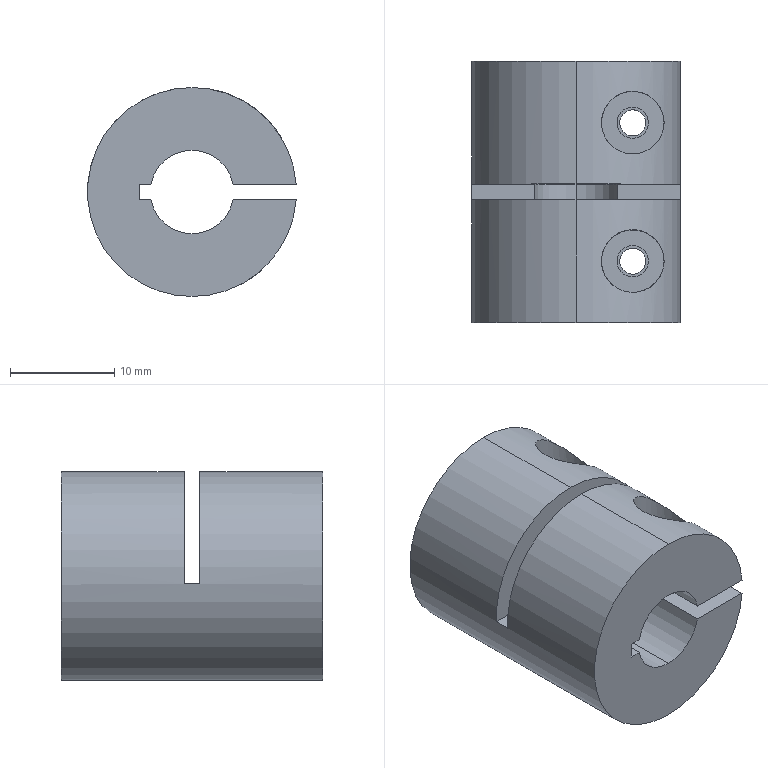Part | SolidWorks | features ICE 4, Extrusion 1, HoleWzd 1 | 1 solid | 34 faces | box 19.972 x 25 x 20 mm | volume 5780 mm3 | cylinder 20 | plane 14 | commonest cylinder face diameters 2.5 x4 3 x4 6 x4 8 x4 20 x4
STEP:
#1=CARTESIAN_POINT('',(4.179,19.125,-9.085));
#2=VERTEX_POINT('',#1);
#3=CARTESIAN_POINT('',(6.679,19.125,-7.442));
#4=VERTEX_POINT('',#3);
#5=CARTESIAN_POINT('',(4.179,19.125,-9.085));
#6=CARTESIAN_POINT('',(4.179,19.034,-9.085));
#7=CARTESIAN_POINT('',(4.189,18.945,-9.08));
#8=CARTESIAN_POINT('',(4.227,18.77,-9.063));
#9=CARTESIAN_POINT('',(4.256,18.684,-9.049));
#10=CARTESIAN_POINT('',(4.33,18.524,-9.014));
#11=CARTESIAN_POINT('',(4.375,18.448,-8.992));
#12=CARTESIAN_POINT('',(4.478,18.309,-8.941));
#13=CARTESIAN_POINT('',(4.536,18.246,-8.912));
#14=CARTESIAN_POINT('',(4.725,18.078,-8.814));
#15=CARTESIAN_POINT('',(4.87,17.996,-8.736));
#16=CARTESIAN_POINT('',(5.169,17.892,-8.562));
#17=CARTESIAN_POINT('',(5.323,17.87,-8.467));
#18=CARTESIAN_POINT('',(5.625,17.881,-8.27));
#19=CARTESIAN_POINT('',(5.772,17.914,-8.168));
#20=CARTESIAN_POINT('',(6.047,18.028,-7.966));
#21=CARTESIAN_POINT('',(6.174,18.11,-7.867));
#22=CARTESIAN_POINT('',(6.344,18.27,-7.73));
#23=CARTESIAN_POINT('',(6.396,18.329,-7.687));
#24=CARTESIAN_POINT('',(6.491,18.46,-7.608));
#25=CARTESIAN_POINT('',(6.533,18.533,-7.571));
#26=CARTESIAN_POINT('',(6.638,18.765,-7.48));
#27=CARTESIAN_POINT('',(6.679,18.943,-7.442));
#28=CARTESIAN_POINT('',(6.679,19.125,-7.442));
#29=B_SPLINE_CURVE_WITH_KNOTS('',3,(#5,#6,#7,#8,#9,#10,#11,#12,#13,#14,#15,#16,#17,#18,#19,#20,#21,#22,#23,#24,#25,#26,#27,#28),.UNSPECIFIED.,.F.,.F.,(4,2,2,2,2,2,2,2,2,2,2,4),(0.004311,0.00458,0.004848,0.005117,0.005385,0.005923,0.00646,0.006997,0.007534,0.007803,0.008071,0.008608),.UNSPECIFIED.);
#30=EDGE_CURVE('',#2,#4,#29,.T.);
#31=ORIENTED_EDGE('',*,*,#30,.F.);
#32=CARTESIAN_POINT('',(4.179,19.125,-0.75));
#33=VERTEX_POINT('',#32);
#34=CARTESIAN_POINT('',(4.179,19.125,-0.75));
#35=DIRECTION('',(0.,0.,1.));
#36=VECTOR('',#35,1000.);
#37=LINE('',#34,#36);
#38=EDGE_CURVE('',#2,#33,#37,.T.);
#39=ORIENTED_EDGE('',*,*,#38,.T.);
#40=CARTESIAN_POINT('',(6.679,19.125,-0.75));
#41=VERTEX_POINT('',#40);
#42=CARTESIAN_POINT('',(5.429,19.125,-0.75));
#43=DIRECTION('',(0.,0.,1.));
#44=DIRECTION('',(1.,0.,0.));
#45=AXIS2_PLACEMENT_3D('',#42,#43,#44);
#46=CIRCLE('',#45,1.25);
#47=EDGE_CURVE('',#33,#41,#46,.T.);
#48=ORIENTED_EDGE('',*,*,#47,.T.);
#49=CARTESIAN_POINT('',(6.679,19.125,-0.75));
#50=DIRECTION('',(0.,0.,1.));
#51=VECTOR('',#50,1000.);
#52=LINE('',#49,#51);
#53=EDGE_CURVE('',#4,#41,#52,.T.);
#54=ORIENTED_EDGE('',*,*,#53,.F.);
#55=EDGE_LOOP('',(#31,#39,#48,#54));
#56=FACE_OUTER_BOUND('',#55,.T.);
#57=CARTESIAN_POINT('',(5.429,19.125,-0.75));
#58=DIRECTION('',(0.,0.,1.));
#59=DIRECTION('',(1.,0.,0.));
#60=AXIS2_PLACEMENT_3D('',#57,#58,#59);
#61=CYLINDRICAL_SURFACE('',#60,1.25);
#62=ADVANCED_FACE('',(#56),#61,.F.);
#63=CARTESIAN_POINT('',(4.179,5.875,-9.085));
#64=VERTEX_POINT('',#63);
#65=CARTESIAN_POINT('',(6.679,5.875,-7.442));
#66=VERTEX_POINT('',#65);
#67=CARTESIAN_POINT('',(4.179,5.875,-9.085));
#68=CARTESIAN_POINT('',(4.179,5.784,-9.085));
#69=CARTESIAN_POINT('',(4.189,5.695,-9.08));
#70=CARTESIAN_POINT('',(4.227,5.52,-9.063));
#71=CARTESIAN_POINT('',(4.256,5.434,-9.049));
#72=CARTESIAN_POINT('',(4.33,5.274,-9.014));
#73=CARTESIAN_POINT('',(4.375,5.198,-8.992));
#74=CARTESIAN_POINT('',(4.478,5.059,-8.941));
#75=CARTESIAN_POINT('',(4.536,4.996,-8.912));
#76=CARTESIAN_POINT('',(4.725,4.828,-8.814));
#77=CARTESIAN_POINT('',(4.87,4.746,-8.736));
#78=CARTESIAN_POINT('',(5.169,4.642,-8.562));
#79=CARTESIAN_POINT('',(5.323,4.62,-8.467));
#80=CARTESIAN_POINT('',(5.625,4.631,-8.27));
#81=CARTESIAN_POINT('',(5.772,4.664,-8.168));
#82=CARTESIAN_POINT('',(6.047,4.778,-7.966));
#83=CARTESIAN_POINT('',(6.174,4.86,-7.867));
#84=CARTESIAN_POINT('',(6.344,5.02,-7.73));
#85=CARTESIAN_POINT('',(6.396,5.079,-7.687));
#86=CARTESIAN_POINT('',(6.491,5.21,-7.608));
#87=CARTESIAN_POINT('',(6.533,5.283,-7.571));
#88=CARTESIAN_POINT('',(6.638,5.515,-7.48));
#89=CARTESIAN_POINT('',(6.679,5.693,-7.442));
#90=CARTESIAN_POINT('',(6.679,5.875,-7.442));
#91=B_SPLINE_CURVE_WITH_KNOTS('',3,(#67,#68,#69,#70,#71,#72,#73,#74,#75,#76,#77,#78,#79,#80,#81,#82,#83,#84,#85,#86,#87,#88,#89,#90),.UNSPECIFIED.,.F.,.F.,(4,2,2,2,2,2,2,2,2,2,2,4),(0.004311,0.00458,0.004848,0.005117,0.005385,0.005923,0.00646,0.006997,0.007534,0.007803,0.008071,0.008608),.UNSPECIFIED.);
#92=EDGE_CURVE('',#64,#66,#91,.T.);
#93=ORIENTED_EDGE('',*,*,#92,.F.);
#94=CARTESIAN_POINT('',(4.179,5.875,-0.75));
#95=VERTEX_POINT('',#94);
#96=CARTESIAN_POINT('',(4.179,5.875,-0.75));
#97=DIRECTION('',(0.,0.,1.));
#98=VECTOR('',#97,1000.);
#99=LINE('',#96,#98);
#100=EDGE_CURVE('',#64,#95,#99,.T.);
#101=ORIENTED_EDGE('',*,*,#100,.T.);
#102=CARTESIAN_POINT('',(6.679,5.875,-0.75));
#103=VERTEX_POINT('',#102);
#104=CARTESIAN_POINT('',(5.429,5.875,-0.75));
#105=DIRECTION('',(0.,0.,1.));
#106=DIRECTION('',(1.,0.,0.));
#107=AXIS2_PLACEMENT_3D('',#104,#105,#106);
#108=CIRCLE('',#107,1.25);
#109=EDGE_CURVE('',#95,#103,#108,.T.);
#110=ORIENTED_EDGE('',*,*,#109,.T.);
#111=CARTESIAN_POINT('',(6.679,5.875,-0.75));
#112=DIRECTION('',(0.,0.,1.));
#113=VECTOR('',#112,1000.);
#114=LINE('',#111,#113);
#115=EDGE_CURVE('',#66,#103,#114,.T.);
#116=ORIENTED_EDGE('',*,*,#115,.F.);
#117=EDGE_LOOP('',(#93,#101,#110,#116));
#118=FACE_OUTER_BOUND('',#117,.T.);
#119=CARTESIAN_POINT('',(5.429,5.875,-0.75));
#120=DIRECTION('',(0.,0.,1.));
#121=DIRECTION('',(1.,0.,0.));
#122=AXIS2_PLACEMENT_3D('',#119,#120,#121);
#123=CYLINDRICAL_SURFACE('',#122,1.25);
#124=ADVANCED_FACE('',(#118),#123,.F.);
#125=CARTESIAN_POINT('',(3.929,19.125,0.75));
#126=VERTEX_POINT('',#125);
#127=CARTESIAN_POINT('',(6.929,19.125,0.75));
#128=VERTEX_POINT('',#127);
#129=CARTESIAN_POINT('',(5.429,19.125,0.75));
#130=DIRECTION('',(0.,0.,1.));
#131=DIRECTION('',(1.,0.,0.));
#132=AXIS2_PLACEMENT_3D('',#129,#130,#131);
#133=CIRCLE('',#132,1.5);
#134=EDGE_CURVE('',#126,#128,#133,.T.);
#135=ORIENTED_EDGE('',*,*,#134,.F.);
#136=CARTESIAN_POINT('',(3.929,19.125,4.));
#137=VERTEX_POINT('',#136);
#138=CARTESIAN_POINT('',(3.929,19.125,0.));
#139=DIRECTION('',(0.,0.,1.));
#140=VECTOR('',#139,1000.);
#141=LINE('',#138,#140);
#142=EDGE_CURVE('',#126,#137,#141,.T.);
#143=ORIENTED_EDGE('',*,*,#142,.T.);
#144=CARTESIAN_POINT('',(6.929,19.125,4.));
#145=VERTEX_POINT('',#144);
#146=CARTESIAN_POINT('',(5.429,19.125,4.));
#147=DIRECTION('',(0.,0.,1.));
#148=DIRECTION('',(1.,0.,0.));
#149=AXIS2_PLACEMENT_3D('',#146,#147,#148);
#150=CIRCLE('',#149,1.5);
#151=EDGE_CURVE('',#137,#145,#150,.T.);
#152=ORIENTED_EDGE('',*,*,#151,.T.);
#153=CARTESIAN_POINT('',(6.929,19.125,0.));
#154=DIRECTION('',(0.,0.,1.));
#155=VECTOR('',#154,1000.);
#156=LINE('',#153,#155);
#157=EDGE_CURVE('',#128,#145,#156,.T.);
#158=ORIENTED_EDGE('',*,*,#157,.F.);
#159=EDGE_LOOP('',(#135,#143,#152,#158));
#160=FACE_OUTER_BOUND('',#159,.T.);
#161=CARTESIAN_POINT('',(5.429,19.125,0.));
#162=DIRECTION('',(0.,0.,1.));
#163=DIRECTION('',(1.,0.,0.));
#164=AXIS2_PLACEMENT_3D('',#161,#162,#163);
#165=CYLINDRICAL_SURFACE('',#164,1.5);
#166=ADVANCED_FACE('',(#160),#165,.F.);
#167=CARTESIAN_POINT('',(3.929,5.875,0.75));
#168=VERTEX_POINT('',#167);
#169=CARTESIAN_POINT('',(6.929,5.875,0.75));
#170=VERTEX_POINT('',#169);
#171=CARTESIAN_POINT('',(5.429,5.875,0.75));
#172=DIRECTION('',(0.,0.,1.));
#173=DIRECTION('',(1.,0.,0.));
#174=AXIS2_PLACEMENT_3D('',#171,#172,#173);
#175=CIRCLE('',#174,1.5);
#176=EDGE_CURVE('',#168,#170,#175,.T.);
#177=ORIENTED_EDGE('',*,*,#176,.F.);
#178=CARTESIAN_POINT('',(3.929,5.875,4.));
#179=VERTEX_POINT('',#178);
#180=CARTESIAN_POINT('',(3.929,5.875,0.));
#181=DIRECTION('',(0.,0.,1.));
#182=VECTOR('',#181,1000.);
#183=LINE('',#180,#182);
#184=EDGE_CURVE('',#168,#179,#183,.T.);
#185=ORIENTED_EDGE('',*,*,#184,.T.);
#186=CARTESIAN_POINT('',(6.929,5.875,4.));
#187=VERTEX_POINT('',#186);
#188=CARTESIAN_POINT('',(5.429,5.875,4.));
#189=DIRECTION('',(0.,0.,1.));
#190=DIRECTION('',(1.,0.,0.));
#191=AXIS2_PLACEMENT_3D('',#188,#189,#190);
#192=CIRCLE('',#191,1.5);
#193=EDGE_CURVE('',#179,#187,#192,.T.);
#194=ORIENTED_EDGE('',*,*,#193,.T.);
#195=CARTESIAN_POINT('',(6.929,5.875,0.));
#196=DIRECTION('',(0.,0.,1.));
#197=VECTOR('',#196,1000.);
#198=LINE('',#195,#197);
#199=EDGE_CURVE('',#170,#187,#198,.T.);
#200=ORIENTED_EDGE('',*,*,#199,.F.);
#201=EDGE_LOOP('',(#177,#185,#194,#200));
#202=FACE_OUTER_BOUND('',#201,.T.);
#203=CARTESIAN_POINT('',(5.429,5.875,0.));
#204=DIRECTION('',(0.,0.,1.));
#205=DIRECTION('',(1.,0.,0.));
#206=AXIS2_PLACEMENT_3D('',#203,#204,#205);
#207=CYLINDRICAL_SURFACE('',#206,1.5);
#208=ADVANCED_FACE('',(#202),#207,.F.);
#209=CARTESIAN_POINT('',(2.429,5.875,4.));
#210=VERTEX_POINT('',#209);
#211=CARTESIAN_POINT('',(8.429,5.875,4.));
#212=VERTEX_POINT('',#211);
#213=CARTESIAN_POINT('',(5.429,5.875,4.));
#214=DIRECTION('',(0.,0.,1.));
#215=DIRECTION('',(-1.,0.,0.));
#216=AXIS2_PLACEMENT_3D('',#213,#214,#215);
#217=CIRCLE('',#216,3.);
#218=EDGE_CURVE('',#210,#212,#217,.T.);
#219=ORIENTED_EDGE('',*,*,#218,.F.);
#220=CARTESIAN_POINT('',(2.429,5.875,9.7));
#221=VERTEX_POINT('',#220);
#222=CARTESIAN_POINT('',(2.429,5.875,4.));
#223=DIRECTION('',(0.,0.,1.));
#224=VECTOR('',#223,1000.);
#225=LINE('',#222,#224);
#226=EDGE_CURVE('',#210,#221,#225,.T.);
#227=ORIENTED_EDGE('',*,*,#226,.T.);
#228=CARTESIAN_POINT('',(8.429,5.875,5.381));
#229=VERTEX_POINT('',#228);
#230=CARTESIAN_POINT('',(8.429,5.875,5.381));
#231=CARTESIAN_POINT('',(8.429,5.65,5.381));
#232=CARTESIAN_POINT('',(8.404,5.431,5.421));
#233=CARTESIAN_POINT('',(8.311,5.016,5.561));
#234=CARTESIAN_POINT('',(8.247,4.827,5.658));
#235=CARTESIAN_POINT('',(8.089,4.474,5.882));
#236=CARTESIAN_POINT('',(7.997,4.314,6.006));
#237=CARTESIAN_POINT('',(7.794,4.021,6.267));
#238=CARTESIAN_POINT('',(7.682,3.887,6.405));
#239=CARTESIAN_POINT('',(7.318,3.519,6.826));
#240=CARTESIAN_POINT('',(7.044,3.324,7.11));
#241=CARTESIAN_POINT('',(6.582,3.1,7.531));
#242=CARTESIAN_POINT('',(6.419,3.037,7.671));
#243=CARTESIAN_POINT('',(6.082,2.942,7.941));
#244=CARTESIAN_POINT('',(5.907,2.908,8.072));
#245=CARTESIAN_POINT('',(5.546,2.872,8.324));
#246=CARTESIAN_POINT('',(5.358,2.87,8.446));
#247=CARTESIAN_POINT('',(4.979,2.903,8.675));
#248=CARTESIAN_POINT('',(4.789,2.937,8.781));
#249=CARTESIAN_POINT('',(4.408,3.047,8.979));
#250=CARTESIAN_POINT('',(4.216,3.124,9.07));
#251=CARTESIAN_POINT('',(3.852,3.314,9.23));
#252=CARTESIAN_POINT('',(3.678,3.43,9.301));
#253=CARTESIAN_POINT('',(3.349,3.703,9.424));
#254=CARTESIAN_POINT('',(3.197,3.859,9.476));
#255=CARTESIAN_POINT('',(2.93,4.201,9.562));
#256=CARTESIAN_POINT('',(2.813,4.39,9.597));
#257=CARTESIAN_POINT('',(2.624,4.789,9.65));
#258=CARTESIAN_POINT('',(2.552,4.997,9.669));
#259=CARTESIAN_POINT('',(2.454,5.431,9.694));
#260=CARTESIAN_POINT('',(2.429,5.654,9.7));
#261=CARTESIAN_POINT('',(2.429,5.875,9.7));
#262=B_SPLINE_CURVE_WITH_KNOTS('',3,(#230,#231,#232,#233,#234,#235,#236,#237,#238,#239,#240,#241,#242,#243,#244,#245,#246,#247,#248,#249,#250,#251,#252,#253,#254,#255,#256,#257,#258,#259,#260,#261),.UNSPECIFIED.,.F.,.F.,(4,2,2,2,2,2,2,2,2,2,2,2,2,2,2,4),(0.,0.0006652,0.00133,0.001995,0.002661,0.003991,0.004656,0.005321,0.005986,0.006652,0.007317,0.007982,0.008647,0.009312,0.009977,0.01064),.UNSPECIFIED.);
#263=EDGE_CURVE('',#229,#221,#262,.T.);
#264=ORIENTED_EDGE('',*,*,#263,.F.);
#265=CARTESIAN_POINT('',(8.429,5.875,4.));
#266=DIRECTION('',(0.,0.,1.));
#267=VECTOR('',#266,1000.);
#268=LINE('',#265,#267);
#269=EDGE_CURVE('',#212,#229,#268,.T.);
#270=ORIENTED_EDGE('',*,*,#269,.F.);
#271=EDGE_LOOP('',(#219,#227,#264,#270));
#272=FACE_OUTER_BOUND('',#271,.T.);
#273=CARTESIAN_POINT('',(5.429,5.875,4.));
#274=DIRECTION('',(0.,0.,1.));
#275=DIRECTION('',(1.,0.,0.));
#276=AXIS2_PLACEMENT_3D('',#273,#274,#275);
#277=CYLINDRICAL_SURFACE('',#276,3.);
#278=ADVANCED_FACE('',(#272),#277,.F.);
#279=CARTESIAN_POINT('',(2.429,19.125,4.));
#280=VERTEX_POINT('',#279);
#281=CARTESIAN_POINT('',(8.429,19.125,4.));
#282=VERTEX_POINT('',#281);
#283=CARTESIAN_POINT('',(5.429,19.125,4.));
#284=DIRECTION('',(0.,0.,1.));
#285=DIRECTION('',(1.,0.,0.));
#286=AXIS2_PLACEMENT_3D('',#283,#284,#285);
#287=CIRCLE('',#286,3.);
#288=EDGE_CURVE('',#280,#282,#287,.T.);
#289=ORIENTED_EDGE('',*,*,#288,.F.);
#290=CARTESIAN_POINT('',(2.429,19.125,9.7));
#291=VERTEX_POINT('',#290);
#292=CARTESIAN_POINT('',(2.429,19.125,4.));
#293=DIRECTION('',(0.,0.,1.));
#294=VECTOR('',#293,1000.);
#295=LINE('',#292,#294);
#296=EDGE_CURVE('',#280,#291,#295,.T.);
#297=ORIENTED_EDGE('',*,*,#296,.T.);
#298=CARTESIAN_POINT('',(8.429,19.125,5.381));
#299=VERTEX_POINT('',#298);
#300=CARTESIAN_POINT('',(8.429,19.125,5.381));
#301=CARTESIAN_POINT('',(8.429,18.9,5.381));
#302=CARTESIAN_POINT('',(8.404,18.681,5.421));
#303=CARTESIAN_POINT('',(8.311,18.266,5.561));
#304=CARTESIAN_POINT('',(8.247,18.077,5.658));
#305=CARTESIAN_POINT('',(8.089,17.724,5.882));
#306=CARTESIAN_POINT('',(7.997,17.564,6.006));
#307=CARTESIAN_POINT('',(7.794,17.271,6.267));
#308=CARTESIAN_POINT('',(7.682,17.137,6.405));
#309=CARTESIAN_POINT('',(7.318,16.769,6.826));
#310=CARTESIAN_POINT('',(7.044,16.574,7.11));
#311=CARTESIAN_POINT('',(6.582,16.35,7.531));
#312=CARTESIAN_POINT('',(6.419,16.287,7.671));
#313=CARTESIAN_POINT('',(6.082,16.192,7.941));
#314=CARTESIAN_POINT('',(5.907,16.158,8.072));
#315=CARTESIAN_POINT('',(5.546,16.122,8.324));
#316=CARTESIAN_POINT('',(5.358,16.12,8.446));
#317=CARTESIAN_POINT('',(4.979,16.153,8.675));
#318=CARTESIAN_POINT('',(4.789,16.187,8.781));
#319=CARTESIAN_POINT('',(4.408,16.297,8.979));
#320=CARTESIAN_POINT('',(4.216,16.374,9.07));
#321=CARTESIAN_POINT('',(3.852,16.564,9.23));
#322=CARTESIAN_POINT('',(3.678,16.68,9.301));
#323=CARTESIAN_POINT('',(3.349,16.953,9.424));
#324=CARTESIAN_POINT('',(3.197,17.109,9.476));
#325=CARTESIAN_POINT('',(2.93,17.451,9.562));
#326=CARTESIAN_POINT('',(2.813,17.64,9.597));
#327=CARTESIAN_POINT('',(2.624,18.039,9.65));
#328=CARTESIAN_POINT('',(2.552,18.247,9.669));
#329=CARTESIAN_POINT('',(2.454,18.681,9.694));
#330=CARTESIAN_POINT('',(2.429,18.904,9.7));
#331=CARTESIAN_POINT('',(2.429,19.125,9.7));
#332=B_SPLINE_CURVE_WITH_KNOTS('',3,(#300,#301,#302,#303,#304,#305,#306,#307,#308,#309,#310,#311,#312,#313,#314,#315,#316,#317,#318,#319,#320,#321,#322,#323,#324,#325,#326,#327,#328,#329,#330,#331),.UNSPECIFIED.,.F.,.F.,(4,2,2,2,2,2,2,2,2,2,2,2,2,2,2,4),(0.,0.0006652,0.00133,0.001995,0.002661,0.003991,0.004656,0.005321,0.005986,0.006652,0.007317,0.007982,0.008647,0.009312,0.009977,0.01064),.UNSPECIFIED.);
#333=EDGE_CURVE('',#299,#291,#332,.T.);
#334=ORIENTED_EDGE('',*,*,#333,.F.);
#335=CARTESIAN_POINT('',(8.429,19.125,4.));
#336=DIRECTION('',(0.,0.,1.));
#337=VECTOR('',#336,1000.);
#338=LINE('',#335,#337);
#339=EDGE_CURVE('',#282,#299,#338,.T.);
#340=ORIENTED_EDGE('',*,*,#339,.F.);
#341=EDGE_LOOP('',(#289,#297,#334,#340));
#342=FACE_OUTER_BOUND('',#341,.T.);
#343=CARTESIAN_POINT('',(5.429,19.125,4.));
#344=DIRECTION('',(0.,0.,1.));
#345=DIRECTION('',(1.,0.,0.));
#346=AXIS2_PLACEMENT_3D('',#343,#344,#345);
#347=CYLINDRICAL_SURFACE('',#346,3.);
#348=ADVANCED_FACE('',(#342),#347,.F.);
#349=ORIENTED_EDGE('',*,*,#333,.T.);
#350=CARTESIAN_POINT('',(2.429,19.125,9.7));
#351=CARTESIAN_POINT('',(2.429,19.346,9.7));
#352=CARTESIAN_POINT('',(2.454,19.569,9.694));
#353=CARTESIAN_POINT('',(2.551,20.001,9.669));
#354=CARTESIAN_POINT('',(2.623,20.209,9.65));
#355=CARTESIAN_POINT('',(2.812,20.608,9.597));
#356=CARTESIAN_POINT('',(2.928,20.796,9.563));
#357=CARTESIAN_POINT('',(3.194,21.138,9.477));
#358=CARTESIAN_POINT('',(3.347,21.295,9.425));
#359=CARTESIAN_POINT('',(3.674,21.567,9.302));
#360=CARTESIAN_POINT('',(3.848,21.683,9.232));
#361=CARTESIAN_POINT('',(4.216,21.877,9.07));
#362=CARTESIAN_POINT('',(4.405,21.952,8.98));
#363=CARTESIAN_POINT('',(4.785,22.062,8.783));
#364=CARTESIAN_POINT('',(4.979,22.097,8.675));
#365=CARTESIAN_POINT('',(5.358,22.13,8.447));
#366=CARTESIAN_POINT('',(5.543,22.128,8.326));
#367=CARTESIAN_POINT('',(5.906,22.093,8.073));
#368=CARTESIAN_POINT('',(6.083,22.058,7.94));
#369=CARTESIAN_POINT('',(6.419,21.962,7.671));
#370=CARTESIAN_POINT('',(6.58,21.901,7.533));
#371=CARTESIAN_POINT('',(6.889,21.751,7.251));
#372=CARTESIAN_POINT('',(7.037,21.664,7.108));
#373=CARTESIAN_POINT('',(7.312,21.467,6.825));
#374=CARTESIAN_POINT('',(7.441,21.357,6.684));
#375=CARTESIAN_POINT('',(7.681,21.114,6.405));
#376=CARTESIAN_POINT('',(7.794,20.979,6.267));
#377=CARTESIAN_POINT('',(7.998,20.684,6.005));
#378=CARTESIAN_POINT('',(8.089,20.525,5.881));
#379=CARTESIAN_POINT('',(8.247,20.173,5.658));
#380=CARTESIAN_POINT('',(8.312,19.982,5.561));
#381=CARTESIAN_POINT('',(8.38,19.673,5.456));
#382=CARTESIAN_POINT('',(8.399,19.565,5.428));
#383=CARTESIAN_POINT('',(8.423,19.348,5.39));
#384=CARTESIAN_POINT('',(8.429,19.237,5.381));
#385=CARTESIAN_POINT('',(8.429,19.125,5.381));
#386=B_SPLINE_CURVE_WITH_KNOTS('',3,(#350,#351,#352,#353,#354,#355,#356,#357,#358,#359,#360,#361,#362,#363,#364,#365,#366,#367,#368,#369,#370,#371,#372,#373,#374,#375,#376,#377,#378,#379,#380,#381,#382,#383,#384,#385),.UNSPECIFIED.,.F.,.F.,(4,2,2,2,2,2,2,2,2,2,2,2,2,2,2,2,2,4),(0.01064,0.01131,0.01197,0.01263,0.0133,0.01396,0.01462,0.01529,0.01595,0.01662,0.01728,0.01794,0.01861,0.01927,0.01993,0.0206,0.02093,0.02126),.UNSPECIFIED.);
#387=EDGE_CURVE('',#291,#299,#386,.T.);
#388=ORIENTED_EDGE('',*,*,#387,.T.);
#389=EDGE_LOOP('',(#349,#388));
#390=FACE_BOUND('',#389,.T.);
#391=CARTESIAN_POINT('',(0.,25.,10.));
#392=VERTEX_POINT('',#391);
#393=CARTESIAN_POINT('',(9.972,25.,0.75));
#394=VERTEX_POINT('',#393);
#395=CARTESIAN_POINT('',(0.,25.,0.));
#396=DIRECTION('',(0.,1.,0.));
#397=DIRECTION('',(0.,0.,1.));
#398=AXIS2_PLACEMENT_3D('',#395,#396,#397);
#399=CIRCLE('',#398,10.);
#400=EDGE_CURVE('',#392,#394,#399,.T.);
#401=ORIENTED_EDGE('',*,*,#400,.F.);
#402=CARTESIAN_POINT('',(0.,13.25,10.));
#403=VERTEX_POINT('',#402);
#404=CARTESIAN_POINT('',(0.,25.,10.));
#405=DIRECTION('',(0.,-1.,0.));
#406=VECTOR('',#405,1000.);
#407=LINE('',#404,#406);
#408=EDGE_CURVE('',#392,#403,#407,.T.);
#409=ORIENTED_EDGE('',*,*,#408,.T.);
#410=CARTESIAN_POINT('',(9.972,13.25,0.75));
#411=VERTEX_POINT('',#410);
#412=CARTESIAN_POINT('',(0.,13.25,0.));
#413=DIRECTION('',(0.,-1.,0.));
#414=DIRECTION('',(0.,0.,-1.));
#415=AXIS2_PLACEMENT_3D('',#412,#413,#414);
#416=CIRCLE('',#415,10.);
#417=EDGE_CURVE('',#411,#403,#416,.T.);
#418=ORIENTED_EDGE('',*,*,#417,.F.);
#419=CARTESIAN_POINT('',(9.972,25.,0.75));
#420=DIRECTION('',(0.,1.,0.));
#421=VECTOR('',#420,1000.);
#422=LINE('',#419,#421);
#423=EDGE_CURVE('',#411,#394,#422,.T.);
#424=ORIENTED_EDGE('',*,*,#423,.T.);
#425=EDGE_LOOP('',(#401,#409,#418,#424));
#426=FACE_OUTER_BOUND('',#425,.T.);
#427=CARTESIAN_POINT('',(0.,25.,0.));
#428=DIRECTION('',(0.,-1.,0.));
#429=DIRECTION('',(0.,0.,-1.));
#430=AXIS2_PLACEMENT_3D('',#427,#428,#429);
#431=CYLINDRICAL_SURFACE('',#430,10.);
#432=ADVANCED_FACE('',(#390,#426),#431,.T.);
#433=ORIENTED_EDGE('',*,*,#263,.T.);
#434=CARTESIAN_POINT('',(2.429,5.875,9.7));
#435=CARTESIAN_POINT('',(2.429,6.096,9.7));
#436=CARTESIAN_POINT('',(2.454,6.319,9.694));
#437=CARTESIAN_POINT('',(2.551,6.751,9.669));
#438=CARTESIAN_POINT('',(2.623,6.959,9.65));
#439=CARTESIAN_POINT('',(2.812,7.358,9.597));
#440=CARTESIAN_POINT('',(2.928,7.546,9.563));
#441=CARTESIAN_POINT('',(3.194,7.888,9.477));
#442=CARTESIAN_POINT('',(3.347,8.045,9.425));
#443=CARTESIAN_POINT('',(3.674,8.317,9.302));
#444=CARTESIAN_POINT('',(3.848,8.433,9.232));
#445=CARTESIAN_POINT('',(4.216,8.627,9.07));
#446=CARTESIAN_POINT('',(4.405,8.702,8.98));
#447=CARTESIAN_POINT('',(4.785,8.812,8.783));
#448=CARTESIAN_POINT('',(4.979,8.847,8.675));
#449=CARTESIAN_POINT('',(5.358,8.88,8.447));
#450=CARTESIAN_POINT('',(5.543,8.878,8.326));
#451=CARTESIAN_POINT('',(5.906,8.843,8.073));
#452=CARTESIAN_POINT('',(6.083,8.808,7.94));
#453=CARTESIAN_POINT('',(6.419,8.712,7.671));
#454=CARTESIAN_POINT('',(6.58,8.651,7.533));
#455=CARTESIAN_POINT('',(6.889,8.501,7.251));
#456=CARTESIAN_POINT('',(7.037,8.414,7.108));
#457=CARTESIAN_POINT('',(7.312,8.217,6.825));
#458=CARTESIAN_POINT('',(7.441,8.107,6.684));
#459=CARTESIAN_POINT('',(7.681,7.864,6.405));
#460=CARTESIAN_POINT('',(7.794,7.729,6.267));
#461=CARTESIAN_POINT('',(7.998,7.434,6.005));
#462=CARTESIAN_POINT('',(8.089,7.275,5.881));
#463=CARTESIAN_POINT('',(8.247,6.923,5.658));
#464=CARTESIAN_POINT('',(8.312,6.732,5.561));
#465=CARTESIAN_POINT('',(8.38,6.423,5.456));
#466=CARTESIAN_POINT('',(8.399,6.315,5.428));
#467=CARTESIAN_POINT('',(8.423,6.098,5.39));
#468=CARTESIAN_POINT('',(8.429,5.987,5.381));
#469=CARTESIAN_POINT('',(8.429,5.875,5.381));
#470=B_SPLINE_CURVE_WITH_KNOTS('',3,(#434,#435,#436,#437,#438,#439,#440,#441,#442,#443,#444,#445,#446,#447,#448,#449,#450,#451,#452,#453,#454,#455,#456,#457,#458,#459,#460,#461,#462,#463,#464,#465,#466,#467,#468,#469),.UNSPECIFIED.,.F.,.F.,(4,2,2,2,2,2,2,2,2,2,2,2,2,2,2,2,2,4),(0.01064,0.01131,0.01197,0.01263,0.0133,0.01396,0.01462,0.01529,0.01595,0.01662,0.01728,0.01794,0.01861,0.01927,0.01993,0.0206,0.02093,0.02126),.UNSPECIFIED.);
#471=EDGE_CURVE('',#221,#229,#470,.T.);
#472=ORIENTED_EDGE('',*,*,#471,.T.);
#473=EDGE_LOOP('',(#433,#472));
#474=FACE_BOUND('',#473,.T.);
#475=CARTESIAN_POINT('',(0.,11.75,10.));
#476=VERTEX_POINT('',#475);
#477=CARTESIAN_POINT('',(9.972,11.75,0.75));
#478=VERTEX_POINT('',#477);
#479=CARTESIAN_POINT('',(0.,11.75,0.));
#480=DIRECTION('',(0.,1.,0.));
#481=DIRECTION('',(0.,0.,1.));
#482=AXIS2_PLACEMENT_3D('',#479,#480,#481);
#483=CIRCLE('',#482,10.);
#484=EDGE_CURVE('',#476,#478,#483,.T.);
#485=ORIENTED_EDGE('',*,*,#484,.F.);
#486=CARTESIAN_POINT('',(0.,0.,10.));
#487=VERTEX_POINT('',#486);
#488=CARTESIAN_POINT('',(0.,25.,10.));
#489=DIRECTION('',(0.,-1.,0.));
#490=VECTOR('',#489,1000.);
#491=LINE('',#488,#490);
#492=EDGE_CURVE('',#476,#487,#491,.T.);
#493=ORIENTED_EDGE('',*,*,#492,.T.);
#494=CARTESIAN_POINT('',(9.972,0.,0.75));
#495=VERTEX_POINT('',#494);
#496=CARTESIAN_POINT('',(0.,0.,0.));
#497=DIRECTION('',(0.,1.,0.));
#498=DIRECTION('',(0.,0.,1.));
#499=AXIS2_PLACEMENT_3D('',#496,#497,#498);
#500=CIRCLE('',#499,10.);
#501=EDGE_CURVE('',#487,#495,#500,.T.);
#502=ORIENTED_EDGE('',*,*,#501,.T.);
#503=CARTESIAN_POINT('',(9.972,25.,0.75));
#504=DIRECTION('',(0.,1.,0.));
#505=VECTOR('',#504,1000.);
#506=LINE('',#503,#505);
#507=EDGE_CURVE('',#495,#478,#506,.T.);
#508=ORIENTED_EDGE('',*,*,#507,.T.);
#509=EDGE_LOOP('',(#485,#493,#502,#508));
#510=FACE_OUTER_BOUND('',#509,.T.);
#511=CARTESIAN_POINT('',(0.,25.,0.));
#512=DIRECTION('',(0.,-1.,0.));
#513=DIRECTION('',(0.,0.,-1.));
#514=AXIS2_PLACEMENT_3D('',#511,#512,#513);
#515=CYLINDRICAL_SURFACE('',#514,10.);
#516=ADVANCED_FACE('',(#474,#510),#515,.T.);
#517=ORIENTED_EDGE('',*,*,#408,.F.);
#518=CARTESIAN_POINT('',(0.,25.,-10.));
#519=VERTEX_POINT('',#518);
#520=CARTESIAN_POINT('',(0.,25.,0.));
#521=DIRECTION('',(0.,1.,0.));
#522=DIRECTION('',(0.,0.,1.));
#523=AXIS2_PLACEMENT_3D('',#520,#521,#522);
#524=CIRCLE('',#523,10.);
#525=EDGE_CURVE('',#519,#392,#524,.T.);
#526=ORIENTED_EDGE('',*,*,#525,.F.);
#527=CARTESIAN_POINT('',(0.,0.,-10.));
#528=VERTEX_POINT('',#527);
#529=CARTESIAN_POINT('',(0.,25.,-10.));
#530=DIRECTION('',(0.,-1.,0.));
#531=VECTOR('',#530,1000.);
#532=LINE('',#529,#531);
#533=EDGE_CURVE('',#519,#528,#532,.T.);
#534=ORIENTED_EDGE('',*,*,#533,.T.);
#535=CARTESIAN_POINT('',(0.,0.,0.));
#536=DIRECTION('',(0.,1.,0.));
#537=DIRECTION('',(0.,0.,1.));
#538=AXIS2_PLACEMENT_3D('',#535,#536,#537);
#539=CIRCLE('',#538,10.);
#540=EDGE_CURVE('',#528,#487,#539,.T.);
#541=ORIENTED_EDGE('',*,*,#540,.T.);
#542=ORIENTED_EDGE('',*,*,#492,.F.);
#543=CARTESIAN_POINT('',(-9.972,11.75,-0.75));
#544=VERTEX_POINT('',#543);
#545=CARTESIAN_POINT('',(0.,11.75,0.));
#546=DIRECTION('',(0.,1.,0.));
#547=DIRECTION('',(0.,0.,1.));
#548=AXIS2_PLACEMENT_3D('',#545,#546,#547);
#549=CIRCLE('',#548,10.);
#550=EDGE_CURVE('',#544,#476,#549,.T.);
#551=ORIENTED_EDGE('',*,*,#550,.F.);
#552=CARTESIAN_POINT('',(-9.972,13.25,-0.75));
#553=VERTEX_POINT('',#552);
#554=CARTESIAN_POINT('',(-9.972,25.,-0.75));
#555=DIRECTION('',(0.,-1.,0.));
#556=VECTOR('',#555,1000.);
#557=LINE('',#554,#556);
#558=EDGE_CURVE('',#553,#544,#557,.T.);
#559=ORIENTED_EDGE('',*,*,#558,.F.);
#560=CARTESIAN_POINT('',(0.,13.25,0.));
#561=DIRECTION('',(0.,-1.,0.));
#562=DIRECTION('',(0.,0.,-1.));
#563=AXIS2_PLACEMENT_3D('',#560,#561,#562);
#564=CIRCLE('',#563,10.);
#565=EDGE_CURVE('',#403,#553,#564,.T.);
#566=ORIENTED_EDGE('',*,*,#565,.F.);
#567=EDGE_LOOP('',(#517,#526,#534,#541,#542,#551,#559,#566));
#568=FACE_OUTER_BOUND('',#567,.T.);
#569=CARTESIAN_POINT('',(0.,25.,0.));
#570=DIRECTION('',(0.,-1.,0.));
#571=DIRECTION('',(0.,0.,-1.));
#572=AXIS2_PLACEMENT_3D('',#569,#570,#571);
#573=CYLINDRICAL_SURFACE('',#572,10.);
#574=ADVANCED_FACE('',(#568),#573,.T.);
#575=CARTESIAN_POINT('',(3.929,25.,-0.75));
#576=VERTEX_POINT('',#575);
#577=CARTESIAN_POINT('',(0.,25.,-4.));
#578=VERTEX_POINT('',#577);
#579=CARTESIAN_POINT('',(0.,25.,0.));
#580=DIRECTION('',(0.,1.,0.));
#581=DIRECTION('',(0.,0.,1.));
#582=AXIS2_PLACEMENT_3D('',#579,#580,#581);
#583=CIRCLE('',#582,4.);
#584=EDGE_CURVE('',#576,#578,#583,.T.);
#585=ORIENTED_EDGE('',*,*,#584,.T.);
#586=CARTESIAN_POINT('',(0.,0.,-4.));
#587=VERTEX_POINT('',#586);
#588=CARTESIAN_POINT('',(0.,25.,-4.));
#589=DIRECTION('',(0.,-1.,0.));
#590=VECTOR('',#589,1000.);
#591=LINE('',#588,#590);
#592=EDGE_CURVE('',#578,#587,#591,.T.);
#593=ORIENTED_EDGE('',*,*,#592,.T.);
#594=CARTESIAN_POINT('',(3.929,0.,-0.75));
#595=VERTEX_POINT('',#594);
#596=CARTESIAN_POINT('',(0.,0.,0.));
#597=DIRECTION('',(0.,1.,0.));
#598=DIRECTION('',(0.,0.,1.));
#599=AXIS2_PLACEMENT_3D('',#596,#597,#598);
#600=CIRCLE('',#599,4.);
#601=EDGE_CURVE('',#595,#587,#600,.T.);
#602=ORIENTED_EDGE('',*,*,#601,.F.);
#603=CARTESIAN_POINT('',(3.929,25.,-0.75));
#604=DIRECTION('',(0.,1.,0.));
#605=VECTOR('',#604,1000.);
#606=LINE('',#603,#605);
#607=EDGE_CURVE('',#595,#576,#606,.T.);
#608=ORIENTED_EDGE('',*,*,#607,.T.);
#609=EDGE_LOOP('',(#585,#593,#602,#608));
#610=FACE_OUTER_BOUND('',#609,.T.);
#611=CARTESIAN_POINT('',(0.,25.,0.));
#612=DIRECTION('',(0.,-1.,0.));
#613=DIRECTION('',(0.,0.,-1.));
#614=AXIS2_PLACEMENT_3D('',#611,#612,#613);
#615=CYLINDRICAL_SURFACE('',#614,4.);
#616=ADVANCED_FACE('',(#610),#615,.F.);
#617=ORIENTED_EDGE('',*,*,#592,.F.);
#618=CARTESIAN_POINT('',(-3.929,25.,-0.75));
#619=VERTEX_POINT('',#618);
#620=CARTESIAN_POINT('',(0.,25.,0.));
#621=DIRECTION('',(0.,1.,0.));
#622=DIRECTION('',(0.,0.,1.));
#623=AXIS2_PLACEMENT_3D('',#620,#621,#622);
#624=CIRCLE('',#623,4.);
#625=EDGE_CURVE('',#578,#619,#624,.T.);
#626=ORIENTED_EDGE('',*,*,#625,.T.);
#627=CARTESIAN_POINT('',(-3.929,0.,-0.75));
#628=VERTEX_POINT('',#627);
#629=CARTESIAN_POINT('',(-3.929,25.,-0.75));
#630=DIRECTION('',(0.,-1.,0.));
#631=VECTOR('',#630,1000.);
#632=LINE('',#629,#631);
#633=EDGE_CURVE('',#619,#628,#632,.T.);
#634=ORIENTED_EDGE('',*,*,#633,.T.);
#635=CARTESIAN_POINT('',(0.,0.,0.));
#636=DIRECTION('',(0.,1.,0.));
#637=DIRECTION('',(0.,0.,1.));
#638=AXIS2_PLACEMENT_3D('',#635,#636,#637);
#639=CIRCLE('',#638,4.);
#640=EDGE_CURVE('',#587,#628,#639,.T.);
#641=ORIENTED_EDGE('',*,*,#640,.F.);
#642=EDGE_LOOP('',(#617,#626,#634,#641));
#643=FACE_OUTER_BOUND('',#642,.T.);
#644=CARTESIAN_POINT('',(0.,25.,0.));
#645=DIRECTION('',(0.,-1.,0.));
#646=DIRECTION('',(0.,0.,-1.));
#647=AXIS2_PLACEMENT_3D('',#644,#645,#646);
#648=CYLINDRICAL_SURFACE('',#647,4.);
#649=ADVANCED_FACE('',(#643),#648,.F.);
#650=CARTESIAN_POINT('',(-3.929,25.,0.75));
#651=VERTEX_POINT('',#650);
#652=CARTESIAN_POINT('',(-3.929,13.25,0.75));
#653=VERTEX_POINT('',#652);
#654=CARTESIAN_POINT('',(-3.929,25.,0.75));
#655=DIRECTION('',(0.,-1.,0.));
#656=VECTOR('',#655,1000.);
#657=LINE('',#654,#656);
#658=EDGE_CURVE('',#651,#653,#657,.T.);
#659=ORIENTED_EDGE('',*,*,#658,.F.);
#660=CARTESIAN_POINT('',(3.929,25.,0.75));
#661=VERTEX_POINT('',#660);
#662=CARTESIAN_POINT('',(0.,25.,0.));
#663=DIRECTION('',(0.,1.,0.));
#664=DIRECTION('',(0.,0.,1.));
#665=AXIS2_PLACEMENT_3D('',#662,#663,#664);
#666=CIRCLE('',#665,4.);
#667=EDGE_CURVE('',#651,#661,#666,.T.);
#668=ORIENTED_EDGE('',*,*,#667,.T.);
#669=CARTESIAN_POINT('',(3.929,25.,0.75));
#670=DIRECTION('',(0.,1.,0.));
#671=VECTOR('',#670,1000.);
#672=LINE('',#669,#671);
#673=EDGE_CURVE('',#126,#661,#672,.T.);
#674=ORIENTED_EDGE('',*,*,#673,.F.);
#675=CARTESIAN_POINT('',(3.929,13.25,0.75));
#676=VERTEX_POINT('',#675);
#677=CARTESIAN_POINT('',(3.929,25.,0.75));
#678=DIRECTION('',(0.,1.,0.));
#679=VECTOR('',#678,1000.);
#680=LINE('',#677,#679);
#681=EDGE_CURVE('',#676,#126,#680,.T.);
#682=ORIENTED_EDGE('',*,*,#681,.F.);
#683=CARTESIAN_POINT('',(0.,13.25,0.));
#684=DIRECTION('',(0.,-1.,0.));
#685=DIRECTION('',(0.,0.,-1.));
#686=AXIS2_PLACEMENT_3D('',#683,#684,#685);
#687=CIRCLE('',#686,4.);
#688=EDGE_CURVE('',#676,#653,#687,.T.);
#689=ORIENTED_EDGE('',*,*,#688,.T.);
#690=EDGE_LOOP('',(#659,#668,#674,#682,#689));
#691=FACE_OUTER_BOUND('',#690,.T.);
#692=CARTESIAN_POINT('',(0.,25.,0.));
#693=DIRECTION('',(0.,-1.,0.));
#694=DIRECTION('',(0.,0.,-1.));
#695=AXIS2_PLACEMENT_3D('',#692,#693,#694);
#696=CYLINDRICAL_SURFACE('',#695,4.);
#697=ADVANCED_FACE('',(#691),#696,.F.);
#698=ORIENTED_EDGE('',*,*,#533,.F.);
#699=CARTESIAN_POINT('',(9.972,25.,-0.75));
#700=VERTEX_POINT('',#699);
#701=CARTESIAN_POINT('',(0.,25.,0.));
#702=DIRECTION('',(0.,1.,0.));
#703=DIRECTION('',(0.,0.,1.));
#704=AXIS2_PLACEMENT_3D('',#701,#702,#703);
#705=CIRCLE('',#704,10.);
#706=EDGE_CURVE('',#700,#519,#705,.T.);
#707=ORIENTED_EDGE('',*,*,#706,.F.);
#708=CARTESIAN_POINT('',(9.972,0.,-0.75));
#709=VERTEX_POINT('',#708);
#710=CARTESIAN_POINT('',(9.972,25.,-0.75));
#711=DIRECTION('',(0.,1.,0.));
#712=VECTOR('',#711,1000.);
#713=LINE('',#710,#712);
#714=EDGE_CURVE('',#709,#700,#713,.T.);
#715=ORIENTED_EDGE('',*,*,#714,.F.);
#716=CARTESIAN_POINT('',(0.,0.,0.));
#717=DIRECTION('',(0.,1.,0.));
#718=DIRECTION('',(0.,0.,1.));
#719=AXIS2_PLACEMENT_3D('',#716,#717,#718);
#720=CIRCLE('',#719,10.);
#721=EDGE_CURVE('',#709,#528,#720,.T.);
#722=ORIENTED_EDGE('',*,*,#721,.T.);
#723=EDGE_LOOP('',(#698,#707,#715,#722));
#724=FACE_OUTER_BOUND('',#723,.T.);
#725=CARTESIAN_POINT('',(6.679,19.125,-7.442));
#726=CARTESIAN_POINT('',(6.679,19.216,-7.442));
#727=CARTESIAN_POINT('',(6.669,19.305,-7.451));
#728=CARTESIAN_POINT('',(6.631,19.479,-7.485));
#729=CARTESIAN_POINT('',(6.603,19.562,-7.51));
#730=CARTESIAN_POINT('',(6.533,19.717,-7.571));
#731=CARTESIAN_POINT('',(6.491,19.79,-7.608));
#732=CARTESIAN_POINT('',(6.396,19.921,-7.687));
#733=CARTESIAN_POINT('',(6.344,19.98,-7.73));
#734=CARTESIAN_POINT('',(6.175,20.14,-7.867));
#735=CARTESIAN_POINT('',(6.046,20.222,-7.967));
#736=CARTESIAN_POINT('',(5.769,20.337,-8.17));
#737=CARTESIAN_POINT('',(5.623,20.369,-8.271));
#738=CARTESIAN_POINT('',(5.321,20.379,-8.469));
#739=CARTESIAN_POINT('',(5.167,20.357,-8.563));
#740=CARTESIAN_POINT('',(4.944,20.28,-8.693));
#741=CARTESIAN_POINT('',(4.87,20.246,-8.734));
#742=CARTESIAN_POINT('',(4.729,20.164,-8.811));
#743=CARTESIAN_POINT('',(4.663,20.116,-8.847));
#744=CARTESIAN_POINT('',(4.538,20.005,-8.911));
#745=CARTESIAN_POINT('',(4.479,19.942,-8.941));
#746=CARTESIAN_POINT('',(4.375,19.803,-8.992));
#747=CARTESIAN_POINT('',(4.331,19.728,-9.014));
#748=CARTESIAN_POINT('',(4.22,19.487,-9.067));
#749=CARTESIAN_POINT('',(4.179,19.307,-9.085));
#750=CARTESIAN_POINT('',(4.179,19.125,-9.085));
#751=B_SPLINE_CURVE_WITH_KNOTS('',3,(#725,#726,#727,#728,#729,#730,#731,#732,#733,#734,#735,#736,#737,#738,#739,#740,#741,#742,#743,#744,#745,#746,#747,#748,#749,#750),.UNSPECIFIED.,.F.,.F.,(4,2,2,2,2,2,2,2,2,2,2,2,4),(0.,0.0002694,0.0005389,0.0008083,0.001078,0.001617,0.002156,0.002694,0.002964,0.003233,0.003503,0.003772,0.004311),.UNSPECIFIED.);
#752=EDGE_CURVE('',#4,#2,#751,.T.);
#753=ORIENTED_EDGE('',*,*,#752,.T.);
#754=ORIENTED_EDGE('',*,*,#30,.T.);
#755=EDGE_LOOP('',(#753,#754));
#756=FACE_BOUND('',#755,.T.);
#757=CARTESIAN_POINT('',(6.679,5.875,-7.442));
#758=CARTESIAN_POINT('',(6.679,5.966,-7.442));
#759=CARTESIAN_POINT('',(6.669,6.055,-7.451));
#760=CARTESIAN_POINT('',(6.631,6.229,-7.485));
#761=CARTESIAN_POINT('',(6.603,6.312,-7.51));
#762=CARTESIAN_POINT('',(6.533,6.467,-7.571));
#763=CARTESIAN_POINT('',(6.491,6.54,-7.608));
#764=CARTESIAN_POINT('',(6.396,6.671,-7.687));
#765=CARTESIAN_POINT('',(6.344,6.73,-7.73));
#766=CARTESIAN_POINT('',(6.175,6.89,-7.867));
#767=CARTESIAN_POINT('',(6.046,6.972,-7.967));
#768=CARTESIAN_POINT('',(5.769,7.087,-8.17));
#769=CARTESIAN_POINT('',(5.623,7.119,-8.271));
#770=CARTESIAN_POINT('',(5.321,7.129,-8.469));
#771=CARTESIAN_POINT('',(5.167,7.107,-8.563));
#772=CARTESIAN_POINT('',(4.944,7.03,-8.693));
#773=CARTESIAN_POINT('',(4.87,6.996,-8.734));
#774=CARTESIAN_POINT('',(4.729,6.914,-8.811));
#775=CARTESIAN_POINT('',(4.663,6.866,-8.847));
#776=CARTESIAN_POINT('',(4.538,6.755,-8.911));
#777=CARTESIAN_POINT('',(4.479,6.692,-8.941));
#778=CARTESIAN_POINT('',(4.375,6.553,-8.992));
#779=CARTESIAN_POINT('',(4.331,6.478,-9.014));
#780=CARTESIAN_POINT('',(4.22,6.237,-9.067));
#781=CARTESIAN_POINT('',(4.179,6.057,-9.085));
#782=CARTESIAN_POINT('',(4.179,5.875,-9.085));
#783=B_SPLINE_CURVE_WITH_KNOTS('',3,(#757,#758,#759,#760,#761,#762,#763,#764,#765,#766,#767,#768,#769,#770,#771,#772,#773,#774,#775,#776,#777,#778,#779,#780,#781,#782),.UNSPECIFIED.,.F.,.F.,(4,2,2,2,2,2,2,2,2,2,2,2,4),(0.,0.0002694,0.0005389,0.0008083,0.001078,0.001617,0.002156,0.002694,0.002964,0.003233,0.003503,0.003772,0.004311),.UNSPECIFIED.);
#784=EDGE_CURVE('',#66,#64,#783,.T.);
#785=ORIENTED_EDGE('',*,*,#784,.T.);
#786=ORIENTED_EDGE('',*,*,#92,.T.);
#787=EDGE_LOOP('',(#785,#786));
#788=FACE_BOUND('',#787,.T.);
#789=CARTESIAN_POINT('',(0.,25.,0.));
#790=DIRECTION('',(0.,-1.,0.));
#791=DIRECTION('',(0.,0.,-1.));
#792=AXIS2_PLACEMENT_3D('',#789,#790,#791);
#793=CYLINDRICAL_SURFACE('',#792,10.);
#794=ADVANCED_FACE('',(#724,#756,#788),#793,.T.);
#795=CARTESIAN_POINT('',(-3.929,11.75,0.75));
#796=VERTEX_POINT('',#795);
#797=CARTESIAN_POINT('',(-3.929,0.,0.75));
#798=VERTEX_POINT('',#797);
#799=CARTESIAN_POINT('',(-3.929,25.,0.75));
#800=DIRECTION('',(0.,-1.,0.));
#801=VECTOR('',#800,1000.);
#802=LINE('',#799,#801);
#803=EDGE_CURVE('',#796,#798,#802,.T.);
#804=ORIENTED_EDGE('',*,*,#803,.F.);
#805=CARTESIAN_POINT('',(3.929,11.75,0.75));
#806=VERTEX_POINT('',#805);
#807=CARTESIAN_POINT('',(0.,11.75,0.));
#808=DIRECTION('',(0.,1.,0.));
#809=DIRECTION('',(0.,0.,1.));
#810=AXIS2_PLACEMENT_3D('',#807,#808,#809);
#811=CIRCLE('',#810,4.);
#812=EDGE_CURVE('',#796,#806,#811,.T.);
#813=ORIENTED_EDGE('',*,*,#812,.T.);
#814=CARTESIAN_POINT('',(3.929,25.,0.75));
#815=DIRECTION('',(0.,1.,0.));
#816=VECTOR('',#815,1000.);
#817=LINE('',#814,#816);
#818=EDGE_CURVE('',#168,#806,#817,.T.);
#819=ORIENTED_EDGE('',*,*,#818,.F.);
#820=CARTESIAN_POINT('',(3.929,0.,0.75));
#821=VERTEX_POINT('',#820);
#822=CARTESIAN_POINT('',(3.929,25.,0.75));
#823=DIRECTION('',(0.,1.,0.));
#824=VECTOR('',#823,1000.);
#825=LINE('',#822,#824);
#826=EDGE_CURVE('',#821,#168,#825,.T.);
#827=ORIENTED_EDGE('',*,*,#826,.F.);
#828=CARTESIAN_POINT('',(0.,0.,0.));
#829=DIRECTION('',(0.,1.,0.));
#830=DIRECTION('',(0.,0.,1.));
#831=AXIS2_PLACEMENT_3D('',#828,#829,#830);
#832=CIRCLE('',#831,4.);
#833=EDGE_CURVE('',#798,#821,#832,.T.);
#834=ORIENTED_EDGE('',*,*,#833,.F.);
#835=EDGE_LOOP('',(#804,#813,#819,#827,#834));
#836=FACE_OUTER_BOUND('',#835,.T.);
#837=CARTESIAN_POINT('',(0.,25.,0.));
#838=DIRECTION('',(0.,-1.,0.));
#839=DIRECTION('',(0.,0.,-1.));
#840=AXIS2_PLACEMENT_3D('',#837,#838,#839);
#841=CYLINDRICAL_SURFACE('',#840,4.);
#842=ADVANCED_FACE('',(#836),#841,.F.);
#843=CARTESIAN_POINT('',(-5.,25.,-0.75));
#844=DIRECTION('',(-1.,0.,0.));
#845=VECTOR('',#844,1000.);
#846=LINE('',#843,#845);
#847=EDGE_CURVE('',#700,#576,#846,.T.);
#848=ORIENTED_EDGE('',*,*,#847,.F.);
#849=ORIENTED_EDGE('',*,*,#706,.T.);
#850=ORIENTED_EDGE('',*,*,#525,.T.);
#851=ORIENTED_EDGE('',*,*,#400,.T.);
#852=CARTESIAN_POINT('',(-5.,25.,0.75));
#853=DIRECTION('',(1.,0.,0.));
#854=VECTOR('',#853,1000.);
#855=LINE('',#852,#854);
#856=EDGE_CURVE('',#661,#394,#855,.T.);
#857=ORIENTED_EDGE('',*,*,#856,.F.);
#858=ORIENTED_EDGE('',*,*,#667,.F.);
#859=CARTESIAN_POINT('',(-5.,25.,0.75));
#860=VERTEX_POINT('',#859);
#861=CARTESIAN_POINT('',(-5.,25.,0.75));
#862=DIRECTION('',(1.,0.,0.));
#863=VECTOR('',#862,1000.);
#864=LINE('',#861,#863);
#865=EDGE_CURVE('',#860,#651,#864,.T.);
#866=ORIENTED_EDGE('',*,*,#865,.F.);
#867=CARTESIAN_POINT('',(-5.,25.,-0.75));
#868=VERTEX_POINT('',#867);
#869=CARTESIAN_POINT('',(-5.,25.,-0.75));
#870=DIRECTION('',(0.,0.,1.));
#871=VECTOR('',#870,1000.);
#872=LINE('',#869,#871);
#873=EDGE_CURVE('',#868,#860,#872,.T.);
#874=ORIENTED_EDGE('',*,*,#873,.F.);
#875=CARTESIAN_POINT('',(-5.,25.,-0.75));
#876=DIRECTION('',(-1.,0.,0.));
#877=VECTOR('',#876,1000.);
#878=LINE('',#875,#877);
#879=EDGE_CURVE('',#619,#868,#878,.T.);
#880=ORIENTED_EDGE('',*,*,#879,.F.);
#881=ORIENTED_EDGE('',*,*,#625,.F.);
#882=ORIENTED_EDGE('',*,*,#584,.F.);
#883=EDGE_LOOP('',(#848,#849,#850,#851,#857,#858,#866,#874,#880,#881,#882));
#884=FACE_OUTER_BOUND('',#883,.T.);
#885=CARTESIAN_POINT('',(0.,25.,0.));
#886=DIRECTION('',(0.,1.,0.));
#887=DIRECTION('',(0.,0.,1.));
#888=AXIS2_PLACEMENT_3D('',#885,#886,#887);
#889=PLANE('',#888);
#890=ADVANCED_FACE('',(#884),#889,.T.);
#891=ORIENTED_EDGE('',*,*,#721,.F.);
#892=CARTESIAN_POINT('',(-5.,0.,-0.75));
#893=DIRECTION('',(-1.,0.,0.));
#894=VECTOR('',#893,1000.);
#895=LINE('',#892,#894);
#896=EDGE_CURVE('',#709,#595,#895,.T.);
#897=ORIENTED_EDGE('',*,*,#896,.T.);
#898=ORIENTED_EDGE('',*,*,#601,.T.);
#899=ORIENTED_EDGE('',*,*,#640,.T.);
#900=CARTESIAN_POINT('',(-5.,0.,-0.75));
#901=VERTEX_POINT('',#900);
#902=CARTESIAN_POINT('',(-5.,0.,-0.75));
#903=DIRECTION('',(-1.,0.,0.));
#904=VECTOR('',#903,1000.);
#905=LINE('',#902,#904);
#906=EDGE_CURVE('',#628,#901,#905,.T.);
#907=ORIENTED_EDGE('',*,*,#906,.T.);
#908=CARTESIAN_POINT('',(-5.,0.,0.75));
#909=VERTEX_POINT('',#908);
#910=CARTESIAN_POINT('',(-5.,0.,-0.75));
#911=DIRECTION('',(0.,0.,1.));
#912=VECTOR('',#911,1000.);
#913=LINE('',#910,#912);
#914=EDGE_CURVE('',#901,#909,#913,.T.);
#915=ORIENTED_EDGE('',*,*,#914,.T.);
#916=CARTESIAN_POINT('',(-5.,0.,0.75));
#917=DIRECTION('',(1.,0.,0.));
#918=VECTOR('',#917,1000.);
#919=LINE('',#916,#918);
#920=EDGE_CURVE('',#909,#798,#919,.T.);
#921=ORIENTED_EDGE('',*,*,#920,.T.);
#922=ORIENTED_EDGE('',*,*,#833,.T.);
#923=CARTESIAN_POINT('',(-5.,0.,0.75));
#924=DIRECTION('',(1.,0.,0.));
#925=VECTOR('',#924,1000.);
#926=LINE('',#923,#925);
#927=EDGE_CURVE('',#821,#495,#926,.T.);
#928=ORIENTED_EDGE('',*,*,#927,.T.);
#929=ORIENTED_EDGE('',*,*,#501,.F.);
#930=ORIENTED_EDGE('',*,*,#540,.F.);
#931=EDGE_LOOP('',(#891,#897,#898,#899,#907,#915,#921,#922,#928,#929,#930));
#932=FACE_OUTER_BOUND('',#931,.T.);
#933=CARTESIAN_POINT('',(0.,0.,0.));
#934=DIRECTION('',(0.,1.,0.));
#935=DIRECTION('',(0.,0.,1.));
#936=AXIS2_PLACEMENT_3D('',#933,#934,#935);
#937=PLANE('',#936);
#938=ADVANCED_FACE('',(#932),#937,.F.);
#939=CARTESIAN_POINT('',(-5.,11.75,-0.75));
#940=VERTEX_POINT('',#939);
#941=CARTESIAN_POINT('',(-5.,11.75,0.75));
#942=VERTEX_POINT('',#941);
#943=CARTESIAN_POINT('',(-5.,11.75,10.));
#944=DIRECTION('',(0.,0.,1.));
#945=VECTOR('',#944,1000.);
#946=LINE('',#943,#945);
#947=EDGE_CURVE('',#940,#942,#946,.T.);
#948=ORIENTED_EDGE('',*,*,#947,.F.);
#949=CARTESIAN_POINT('',(25.,11.75,-0.75));
#950=DIRECTION('',(-1.,0.,0.));
#951=VECTOR('',#950,1000.);
#952=LINE('',#949,#951);
#953=EDGE_CURVE('',#940,#544,#952,.T.);
#954=ORIENTED_EDGE('',*,*,#953,.T.);
#955=ORIENTED_EDGE('',*,*,#550,.T.);
#956=ORIENTED_EDGE('',*,*,#484,.T.);
#957=CARTESIAN_POINT('',(25.,11.75,0.75));
#958=DIRECTION('',(1.,0.,0.));
#959=VECTOR('',#958,1000.);
#960=LINE('',#957,#959);
#961=EDGE_CURVE('',#806,#478,#960,.T.);
#962=ORIENTED_EDGE('',*,*,#961,.F.);
#963=ORIENTED_EDGE('',*,*,#812,.F.);
#964=CARTESIAN_POINT('',(25.,11.75,0.75));
#965=DIRECTION('',(1.,0.,0.));
#966=VECTOR('',#965,1000.);
#967=LINE('',#964,#966);
#968=EDGE_CURVE('',#942,#796,#967,.T.);
#969=ORIENTED_EDGE('',*,*,#968,.F.);
#970=EDGE_LOOP('',(#948,#954,#955,#956,#962,#963,#969));
#971=FACE_OUTER_BOUND('',#970,.T.);
#972=CARTESIAN_POINT('',(25.,11.75,10.));
#973=DIRECTION('',(0.,1.,0.));
#974=DIRECTION('',(0.,0.,1.));
#975=AXIS2_PLACEMENT_3D('',#972,#973,#974);
#976=PLANE('',#975);
#977=ADVANCED_FACE('',(#971),#976,.T.);
#978=ORIENTED_EDGE('',*,*,#953,.F.);
#979=CARTESIAN_POINT('',(-5.,0.,-0.75));
#980=DIRECTION('',(0.,1.,0.));
#981=VECTOR('',#980,1000.);
#982=LINE('',#979,#981);
#983=EDGE_CURVE('',#901,#940,#982,.T.);
#984=ORIENTED_EDGE('',*,*,#983,.F.);
#985=ORIENTED_EDGE('',*,*,#906,.F.);
#986=ORIENTED_EDGE('',*,*,#633,.F.);
#987=ORIENTED_EDGE('',*,*,#879,.T.);
#988=CARTESIAN_POINT('',(-5.,13.25,-0.75));
#989=VERTEX_POINT('',#988);
#990=CARTESIAN_POINT('',(-5.,0.,-0.75));
#991=DIRECTION('',(0.,1.,0.));
#992=VECTOR('',#991,1000.);
#993=LINE('',#990,#992);
#994=EDGE_CURVE('',#989,#868,#993,.T.);
#995=ORIENTED_EDGE('',*,*,#994,.F.);
#996=CARTESIAN_POINT('',(25.,13.25,-0.75));
#997=DIRECTION('',(-1.,0.,0.));
#998=VECTOR('',#997,1000.);
#999=LINE('',#996,#998);
#1000=EDGE_CURVE('',#989,#553,#999,.T.);
#1001=ORIENTED_EDGE('',*,*,#1000,.T.);
#1002=ORIENTED_EDGE('',*,*,#558,.T.);
#1003=EDGE_LOOP('',(#978,#984,#985,#986,#987,#995,#1001,#1002));
#1004=FACE_OUTER_BOUND('',#1003,.T.);
#1005=CARTESIAN_POINT('',(25.,13.25,-0.75));
#1006=DIRECTION('',(0.,0.,1.));
#1007=DIRECTION('',(0.,-1.,0.));
#1008=AXIS2_PLACEMENT_3D('',#1005,#1006,#1007);
#1009=PLANE('',#1008);
#1010=ADVANCED_FACE('',(#1004),#1009,.T.);
#1011=CARTESIAN_POINT('',(5.429,19.125,-0.75));
#1012=DIRECTION('',(0.,0.,1.));
#1013=DIRECTION('',(1.,0.,0.));
#1014=AXIS2_PLACEMENT_3D('',#1011,#1012,#1013);
#1015=CIRCLE('',#1014,1.25);
#1016=EDGE_CURVE('',#41,#33,#1015,.T.);
#1017=ORIENTED_EDGE('',*,*,#1016,.F.);
#1018=ORIENTED_EDGE('',*,*,#47,.F.);
#1019=EDGE_LOOP('',(#1017,#1018));
#1020=FACE_BOUND('',#1019,.T.);
#1021=CARTESIAN_POINT('',(5.429,5.875,-0.75));
#1022=DIRECTION('',(0.,0.,1.));
#1023=DIRECTION('',(1.,0.,0.));
#1024=AXIS2_PLACEMENT_3D('',#1021,#1022,#1023);
#1025=CIRCLE('',#1024,1.25);
#1026=EDGE_CURVE('',#103,#95,#1025,.T.);
#1027=ORIENTED_EDGE('',*,*,#1026,.F.);
#1028=ORIENTED_EDGE('',*,*,#109,.F.);
#1029=EDGE_LOOP('',(#1027,#1028));
#1030=FACE_BOUND('',#1029,.T.);
#1031=ORIENTED_EDGE('',*,*,#714,.T.);
#1032=ORIENTED_EDGE('',*,*,#847,.T.);
#1033=ORIENTED_EDGE('',*,*,#607,.F.);
#1034=ORIENTED_EDGE('',*,*,#896,.F.);
#1035=EDGE_LOOP('',(#1031,#1032,#1033,#1034));
#1036=FACE_OUTER_BOUND('',#1035,.T.);
#1037=CARTESIAN_POINT('',(25.,13.25,-0.75));
#1038=DIRECTION('',(0.,0.,1.));
#1039=DIRECTION('',(0.,-1.,0.));
#1040=AXIS2_PLACEMENT_3D('',#1037,#1038,#1039);
#1041=PLANE('',#1040);
#1042=ADVANCED_FACE('',(#1020,#1030,#1036),#1041,.T.);
#1043=CARTESIAN_POINT('',(25.,13.25,0.75));
#1044=DIRECTION('',(-1.,0.,0.));
#1045=VECTOR('',#1044,1000.);
#1046=LINE('',#1043,#1045);
#1047=EDGE_CURVE('',#411,#676,#1046,.T.);
#1048=ORIENTED_EDGE('',*,*,#1047,.F.);
#1049=ORIENTED_EDGE('',*,*,#417,.T.);
#1050=ORIENTED_EDGE('',*,*,#565,.T.);
#1051=ORIENTED_EDGE('',*,*,#1000,.F.);
#1052=CARTESIAN_POINT('',(-5.,13.25,0.75));
#1053=VERTEX_POINT('',#1052);
#1054=CARTESIAN_POINT('',(-5.,13.25,10.));
#1055=DIRECTION('',(0.,0.,-1.));
#1056=VECTOR('',#1055,1000.);
#1057=LINE('',#1054,#1056);
#1058=EDGE_CURVE('',#1053,#989,#1057,.T.);
#1059=ORIENTED_EDGE('',*,*,#1058,.F.);
#1060=CARTESIAN_POINT('',(25.,13.25,0.75));
#1061=DIRECTION('',(-1.,0.,0.));
#1062=VECTOR('',#1061,1000.);
#1063=LINE('',#1060,#1062);
#1064=EDGE_CURVE('',#653,#1053,#1063,.T.);
#1065=ORIENTED_EDGE('',*,*,#1064,.F.);
#1066=ORIENTED_EDGE('',*,*,#688,.F.);
#1067=EDGE_LOOP('',(#1048,#1049,#1050,#1051,#1059,#1065,#1066));
#1068=FACE_OUTER_BOUND('',#1067,.T.);
#1069=CARTESIAN_POINT('',(25.,13.25,10.));
#1070=DIRECTION('',(0.,-1.,0.));
#1071=DIRECTION('',(0.,0.,-1.));
#1072=AXIS2_PLACEMENT_3D('',#1069,#1070,#1071);
#1073=PLANE('',#1072);
#1074=ADVANCED_FACE('',(#1068),#1073,.T.);
#1075=ORIENTED_EDGE('',*,*,#658,.T.);
#1076=ORIENTED_EDGE('',*,*,#1064,.T.);
#1077=CARTESIAN_POINT('',(-5.,0.,0.75));
#1078=DIRECTION('',(0.,1.,0.));
#1079=VECTOR('',#1078,1000.);
#1080=LINE('',#1077,#1079);
#1081=EDGE_CURVE('',#1053,#860,#1080,.T.);
#1082=ORIENTED_EDGE('',*,*,#1081,.T.);
#1083=ORIENTED_EDGE('',*,*,#865,.T.);
#1084=EDGE_LOOP('',(#1075,#1076,#1082,#1083));
#1085=FACE_OUTER_BOUND('',#1084,.T.);
#1086=CARTESIAN_POINT('',(-5.,0.,0.75));
#1087=DIRECTION('',(0.,0.,1.));
#1088=DIRECTION('',(1.,0.,0.));
#1089=AXIS2_PLACEMENT_3D('',#1086,#1087,#1088);
#1090=PLANE('',#1089);
#1091=ADVANCED_FACE('',(#1085),#1090,.F.);
#1092=ORIENTED_EDGE('',*,*,#1058,.T.);
#1093=ORIENTED_EDGE('',*,*,#994,.T.);
#1094=ORIENTED_EDGE('',*,*,#873,.T.);
#1095=ORIENTED_EDGE('',*,*,#1081,.F.);
#1096=EDGE_LOOP('',(#1092,#1093,#1094,#1095));
#1097=FACE_OUTER_BOUND('',#1096,.T.);
#1098=CARTESIAN_POINT('',(-5.,0.,-0.75));
#1099=DIRECTION('',(-1.,0.,0.));
#1100=DIRECTION('',(0.,0.,1.));
#1101=AXIS2_PLACEMENT_3D('',#1098,#1099,#1100);
#1102=PLANE('',#1101);
#1103=ADVANCED_FACE('',(#1097),#1102,.F.);
#1104=ORIENTED_EDGE('',*,*,#681,.T.);
#1105=ORIENTED_EDGE('',*,*,#134,.T.);
#1106=CARTESIAN_POINT('',(5.429,19.125,0.75));
#1107=DIRECTION('',(0.,0.,1.));
#1108=DIRECTION('',(1.,0.,0.));
#1109=AXIS2_PLACEMENT_3D('',#1106,#1107,#1108);
#1110=CIRCLE('',#1109,1.5);
#1111=EDGE_CURVE('',#128,#126,#1110,.T.);
#1112=ORIENTED_EDGE('',*,*,#1111,.T.);
#1113=ORIENTED_EDGE('',*,*,#673,.T.);
#1114=ORIENTED_EDGE('',*,*,#856,.T.);
#1115=ORIENTED_EDGE('',*,*,#423,.F.);
#1116=ORIENTED_EDGE('',*,*,#1047,.T.);
#1117=EDGE_LOOP('',(#1104,#1105,#1112,#1113,#1114,#1115,#1116));
#1118=FACE_OUTER_BOUND('',#1117,.T.);
#1119=CARTESIAN_POINT('',(-5.,0.,0.75));
#1120=DIRECTION('',(0.,0.,1.));
#1121=DIRECTION('',(1.,0.,0.));
#1122=AXIS2_PLACEMENT_3D('',#1119,#1120,#1121);
#1123=PLANE('',#1122);
#1124=ADVANCED_FACE('',(#1118),#1123,.F.);
#1125=ORIENTED_EDGE('',*,*,#826,.T.);
#1126=ORIENTED_EDGE('',*,*,#176,.T.);
#1127=CARTESIAN_POINT('',(5.429,5.875,0.75));
#1128=DIRECTION('',(0.,0.,1.));
#1129=DIRECTION('',(1.,0.,0.));
#1130=AXIS2_PLACEMENT_3D('',#1127,#1128,#1129);
#1131=CIRCLE('',#1130,1.5);
#1132=EDGE_CURVE('',#170,#168,#1131,.T.);
#1133=ORIENTED_EDGE('',*,*,#1132,.T.);
#1134=ORIENTED_EDGE('',*,*,#818,.T.);
#1135=ORIENTED_EDGE('',*,*,#961,.T.);
#1136=ORIENTED_EDGE('',*,*,#507,.F.);
#1137=ORIENTED_EDGE('',*,*,#927,.F.);
#1138=EDGE_LOOP('',(#1125,#1126,#1133,#1134,#1135,#1136,#1137));
#1139=FACE_OUTER_BOUND('',#1138,.T.);
#1140=CARTESIAN_POINT('',(-5.,0.,0.75));
#1141=DIRECTION('',(0.,0.,1.));
#1142=DIRECTION('',(1.,0.,0.));
#1143=AXIS2_PLACEMENT_3D('',#1140,#1141,#1142);
#1144=PLANE('',#1143);
#1145=ADVANCED_FACE('',(#1139),#1144,.F.);
#1146=ORIENTED_EDGE('',*,*,#803,.T.);
#1147=ORIENTED_EDGE('',*,*,#920,.F.);
#1148=CARTESIAN_POINT('',(-5.,0.,0.75));
#1149=DIRECTION('',(0.,1.,0.));
#1150=VECTOR('',#1149,1000.);
#1151=LINE('',#1148,#1150);
#1152=EDGE_CURVE('',#909,#942,#1151,.T.);
#1153=ORIENTED_EDGE('',*,*,#1152,.T.);
#1154=ORIENTED_EDGE('',*,*,#968,.T.);
#1155=EDGE_LOOP('',(#1146,#1147,#1153,#1154));
#1156=FACE_OUTER_BOUND('',#1155,.T.);
#1157=CARTESIAN_POINT('',(-5.,0.,0.75));
#1158=DIRECTION('',(0.,0.,1.));
#1159=DIRECTION('',(1.,0.,0.));
#1160=AXIS2_PLACEMENT_3D('',#1157,#1158,#1159);
#1161=PLANE('',#1160);
#1162=ADVANCED_FACE('',(#1156),#1161,.F.);
#1163=ORIENTED_EDGE('',*,*,#947,.T.);
#1164=ORIENTED_EDGE('',*,*,#1152,.F.);
#1165=ORIENTED_EDGE('',*,*,#914,.F.);
#1166=ORIENTED_EDGE('',*,*,#983,.T.);
#1167=EDGE_LOOP('',(#1163,#1164,#1165,#1166));
#1168=FACE_OUTER_BOUND('',#1167,.T.);
#1169=CARTESIAN_POINT('',(-5.,0.,-0.75));
#1170=DIRECTION('',(-1.,0.,0.));
#1171=DIRECTION('',(0.,0.,1.));
#1172=AXIS2_PLACEMENT_3D('',#1169,#1170,#1171);
#1173=PLANE('',#1172);
#1174=ADVANCED_FACE('',(#1168),#1173,.F.);
#1175=ORIENTED_EDGE('',*,*,#296,.F.);
#1176=CARTESIAN_POINT('',(5.429,19.125,4.));
#1177=DIRECTION('',(0.,0.,1.));
#1178=DIRECTION('',(1.,0.,0.));
#1179=AXIS2_PLACEMENT_3D('',#1176,#1177,#1178);
#1180=CIRCLE('',#1179,3.);
#1181=EDGE_CURVE('',#282,#280,#1180,.T.);
#1182=ORIENTED_EDGE('',*,*,#1181,.F.);
#1183=ORIENTED_EDGE('',*,*,#339,.T.);
#1184=ORIENTED_EDGE('',*,*,#387,.F.);
#1185=EDGE_LOOP('',(#1175,#1182,#1183,#1184));
#1186=FACE_OUTER_BOUND('',#1185,.T.);
#1187=CARTESIAN_POINT('',(5.429,19.125,4.));
#1188=DIRECTION('',(0.,0.,1.));
#1189=DIRECTION('',(1.,0.,0.));
#1190=AXIS2_PLACEMENT_3D('',#1187,#1188,#1189);
#1191=CYLINDRICAL_SURFACE('',#1190,3.);
#1192=ADVANCED_FACE('',(#1186),#1191,.F.);
#1193=CARTESIAN_POINT('',(5.429,19.125,4.));
#1194=DIRECTION('',(0.,0.,1.));
#1195=DIRECTION('',(1.,0.,0.));
#1196=AXIS2_PLACEMENT_3D('',#1193,#1194,#1195);
#1197=CIRCLE('',#1196,1.5);
#1198=EDGE_CURVE('',#145,#137,#1197,.T.);
#1199=ORIENTED_EDGE('',*,*,#1198,.F.);
#1200=ORIENTED_EDGE('',*,*,#151,.F.);
#1201=EDGE_LOOP('',(#1199,#1200));
#1202=FACE_BOUND('',#1201,.T.);
#1203=ORIENTED_EDGE('',*,*,#1181,.T.);
#1204=ORIENTED_EDGE('',*,*,#288,.T.);
#1205=EDGE_LOOP('',(#1203,#1204));
#1206=FACE_OUTER_BOUND('',#1205,.T.);
#1207=CARTESIAN_POINT('',(5.429,19.125,4.));
#1208=DIRECTION('',(0.,0.,1.));
#1209=DIRECTION('',(1.,0.,0.));
#1210=AXIS2_PLACEMENT_3D('',#1207,#1208,#1209);
#1211=PLANE('',#1210);
#1212=ADVANCED_FACE('',(#1202,#1206),#1211,.T.);
#1213=ORIENTED_EDGE('',*,*,#226,.F.);
#1214=CARTESIAN_POINT('',(5.429,5.875,4.));
#1215=DIRECTION('',(0.,0.,1.));
#1216=DIRECTION('',(-1.,0.,0.));
#1217=AXIS2_PLACEMENT_3D('',#1214,#1215,#1216);
#1218=CIRCLE('',#1217,3.);
#1219=EDGE_CURVE('',#212,#210,#1218,.T.);
#1220=ORIENTED_EDGE('',*,*,#1219,.F.);
#1221=ORIENTED_EDGE('',*,*,#269,.T.);
#1222=ORIENTED_EDGE('',*,*,#471,.F.);
#1223=EDGE_LOOP('',(#1213,#1220,#1221,#1222));
#1224=FACE_OUTER_BOUND('',#1223,.T.);
#1225=CARTESIAN_POINT('',(5.429,5.875,4.));
#1226=DIRECTION('',(0.,0.,1.));
#1227=DIRECTION('',(1.,0.,0.));
#1228=AXIS2_PLACEMENT_3D('',#1225,#1226,#1227);
#1229=CYLINDRICAL_SURFACE('',#1228,3.);
#1230=ADVANCED_FACE('',(#1224),#1229,.F.);
#1231=CARTESIAN_POINT('',(5.429,5.875,4.));
#1232=DIRECTION('',(0.,0.,1.));
#1233=DIRECTION('',(1.,0.,0.));
#1234=AXIS2_PLACEMENT_3D('',#1231,#1232,#1233);
#1235=CIRCLE('',#1234,1.5);
#1236=EDGE_CURVE('',#187,#179,#1235,.T.);
#1237=ORIENTED_EDGE('',*,*,#1236,.F.);
#1238=ORIENTED_EDGE('',*,*,#193,.F.);
#1239=EDGE_LOOP('',(#1237,#1238));
#1240=FACE_BOUND('',#1239,.T.);
#1241=ORIENTED_EDGE('',*,*,#1219,.T.);
#1242=ORIENTED_EDGE('',*,*,#218,.T.);
#1243=EDGE_LOOP('',(#1241,#1242));
#1244=FACE_OUTER_BOUND('',#1243,.T.);
#1245=CARTESIAN_POINT('',(5.429,5.875,4.));
#1246=DIRECTION('',(0.,0.,-1.));
#1247=DIRECTION('',(-1.,0.,0.));
#1248=AXIS2_PLACEMENT_3D('',#1245,#1246,#1247);
#1249=PLANE('',#1248);
#1250=ADVANCED_FACE('',(#1240,#1244),#1249,.F.);
#1251=ORIENTED_EDGE('',*,*,#184,.F.);
#1252=ORIENTED_EDGE('',*,*,#1132,.F.);
#1253=ORIENTED_EDGE('',*,*,#199,.T.);
#1254=ORIENTED_EDGE('',*,*,#1236,.T.);
#1255=EDGE_LOOP('',(#1251,#1252,#1253,#1254));
#1256=FACE_OUTER_BOUND('',#1255,.T.);
#1257=CARTESIAN_POINT('',(5.429,5.875,0.));
#1258=DIRECTION('',(0.,0.,1.));
#1259=DIRECTION('',(1.,0.,0.));
#1260=AXIS2_PLACEMENT_3D('',#1257,#1258,#1259);
#1261=CYLINDRICAL_SURFACE('',#1260,1.5);
#1262=ADVANCED_FACE('',(#1256),#1261,.F.);
#1263=ORIENTED_EDGE('',*,*,#142,.F.);
#1264=ORIENTED_EDGE('',*,*,#1111,.F.);
#1265=ORIENTED_EDGE('',*,*,#157,.T.);
#1266=ORIENTED_EDGE('',*,*,#1198,.T.);
#1267=EDGE_LOOP('',(#1263,#1264,#1265,#1266));
#1268=FACE_OUTER_BOUND('',#1267,.T.);
#1269=CARTESIAN_POINT('',(5.429,19.125,0.));
#1270=DIRECTION('',(0.,0.,1.));
#1271=DIRECTION('',(1.,0.,0.));
#1272=AXIS2_PLACEMENT_3D('',#1269,#1270,#1271);
#1273=CYLINDRICAL_SURFACE('',#1272,1.5);
#1274=ADVANCED_FACE('',(#1268),#1273,.F.);
#1275=ORIENTED_EDGE('',*,*,#100,.F.);
#1276=ORIENTED_EDGE('',*,*,#784,.F.);
#1277=ORIENTED_EDGE('',*,*,#115,.T.);
#1278=ORIENTED_EDGE('',*,*,#1026,.T.);
#1279=EDGE_LOOP('',(#1275,#1276,#1277,#1278));
#1280=FACE_OUTER_BOUND('',#1279,.T.);
#1281=CARTESIAN_POINT('',(5.429,5.875,-0.75));
#1282=DIRECTION('',(0.,0.,1.));
#1283=DIRECTION('',(1.,0.,0.));
#1284=AXIS2_PLACEMENT_3D('',#1281,#1282,#1283);
#1285=CYLINDRICAL_SURFACE('',#1284,1.25);
#1286=ADVANCED_FACE('',(#1280),#1285,.F.);
#1287=ORIENTED_EDGE('',*,*,#38,.F.);
#1288=ORIENTED_EDGE('',*,*,#752,.F.);
#1289=ORIENTED_EDGE('',*,*,#53,.T.);
#1290=ORIENTED_EDGE('',*,*,#1016,.T.);
#1291=EDGE_LOOP('',(#1287,#1288,#1289,#1290));
#1292=FACE_OUTER_BOUND('',#1291,.T.);
#1293=CARTESIAN_POINT('',(5.429,19.125,-0.75));
#1294=DIRECTION('',(0.,0.,1.));
#1295=DIRECTION('',(1.,0.,0.));
#1296=AXIS2_PLACEMENT_3D('',#1293,#1294,#1295);
#1297=CYLINDRICAL_SURFACE('',#1296,1.25);
#1298=ADVANCED_FACE('',(#1292),#1297,.F.);
#1299=CLOSED_SHELL('',(#62,#124,#166,#208,#278,#348,#432,#516,#574,#616,#649,#697,#794,#842,#890,#938,#977,#1010,#1042,#1074,#1091,#1103,#1124,#1145,#1162,#1174,#1192,#1212,#1230,#1250,#1262,#1274,#1286,#1298));
#1300=MANIFOLD_SOLID_BREP('',#1299);
#1301=CARTESIAN_POINT('',(0.,0.,0.));
#1302=DIRECTION('',(0.,0.,1.));
#1303=DIRECTION('',(1.,0.,0.));
#1304=AXIS2_PLACEMENT_3D('',#1301,#1302,#1303);
#1305=(LENGTH_UNIT()NAMED_UNIT(*)SI_UNIT(.MILLI.,.METRE.));
#1306=UNCERTAINTY_MEASURE_WITH_UNIT(LENGTH_MEASURE(0.00001),#1305,'','');
#1307=(NAMED_UNIT(*)PLANE_ANGLE_UNIT()SI_UNIT($,.RADIAN.));
#1308=(NAMED_UNIT(*)SI_UNIT($,.STERADIAN.)SOLID_ANGLE_UNIT());
#1309=(GEOMETRIC_REPRESENTATION_CONTEXT(3)GLOBAL_UNCERTAINTY_ASSIGNED_CONTEXT((#1306))GLOBAL_UNIT_ASSIGNED_CONTEXT((#1305,#1307,#1308))REPRESENTATION_CONTEXT('',''));
#1310=ADVANCED_BREP_SHAPE_REPRESENTATION('',(#1300,#1304),#1309);